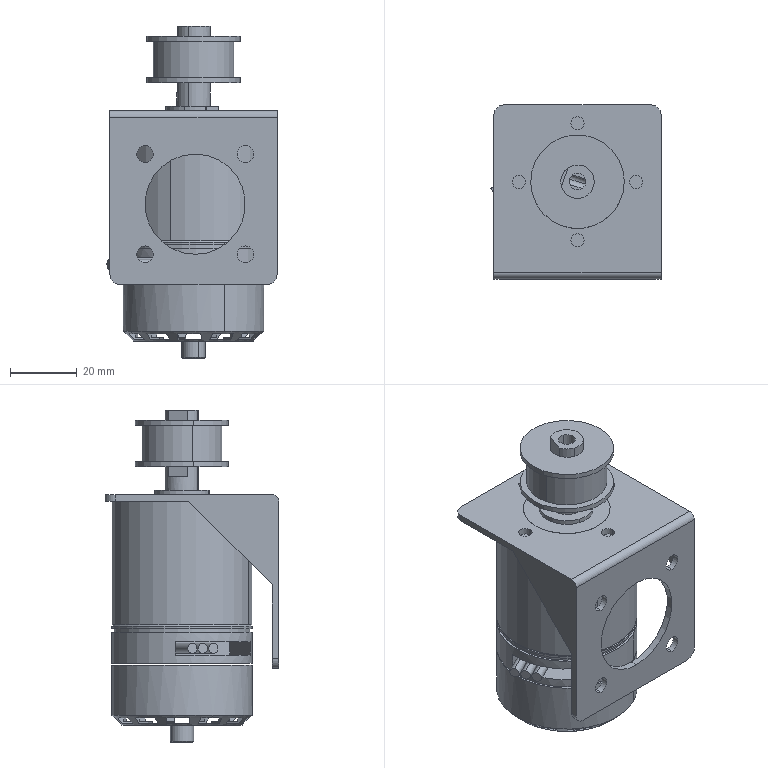Part | SolidWorks | 6 solids | 252 faces | box 50.9 x 52 x 99.3 mm | volume 89740 mm3 | plane 137 | cylinder 107 | cone 8 | commonest cylinder face diameters 4 x25 3 x20 5 x18 42 x8 10 x7 6 x4